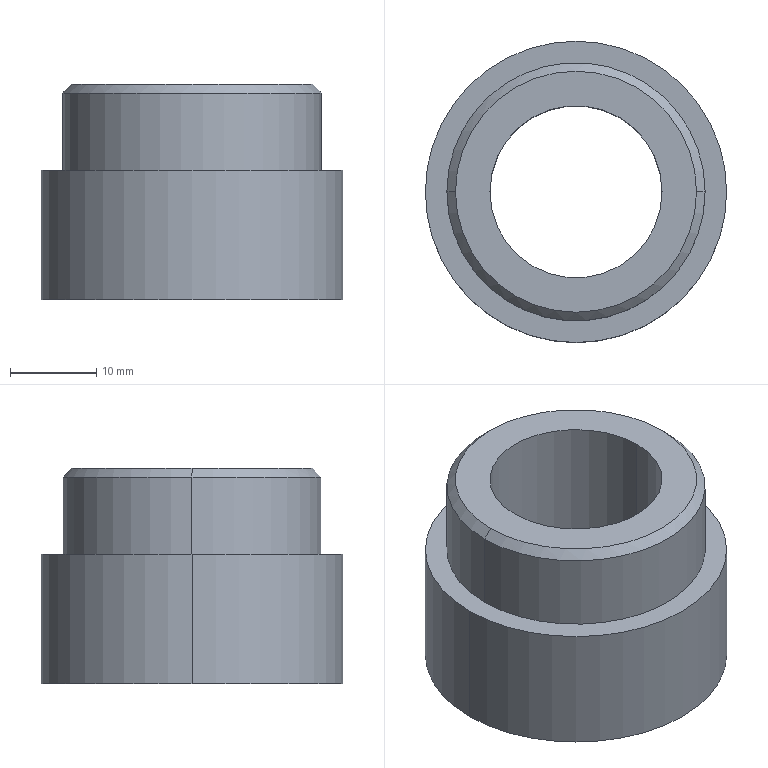Part | SolidWorks | features Chamfer 1, Extrusion 1, ICE 1 | 1 solid | 11 faces | box 35 x 35 x 25 mm | volume 13600 mm3 | cylinder 6 | plane 3 | cone 2 | commonest cylinder face diameters 20 x2 30 x2 35 x2
STEP:
#1=CARTESIAN_POINT('',(14.,0.,25.));
#2=VERTEX_POINT('',#1);
#3=CARTESIAN_POINT('',(-14.,0.,25.));
#4=VERTEX_POINT('',#3);
#5=CARTESIAN_POINT('',(0.,0.,25.));
#6=DIRECTION('',(0.,0.,1.));
#7=DIRECTION('',(1.,0.,0.));
#8=AXIS2_PLACEMENT_3D('',#5,#6,#7);
#9=CIRCLE('',#8,14.);
#10=EDGE_CURVE('',#2,#4,#9,.T.);
#11=ORIENTED_EDGE('',*,*,#10,.F.);
#12=CARTESIAN_POINT('',(15.,0.,24.));
#13=VERTEX_POINT('',#12);
#14=CARTESIAN_POINT('',(14.,0.,25.));
#15=DIRECTION('',(0.7071,0.,-0.7071));
#16=VECTOR('',#15,1000.);
#17=LINE('',#14,#16);
#18=EDGE_CURVE('',#2,#13,#17,.T.);
#19=ORIENTED_EDGE('',*,*,#18,.T.);
#20=CARTESIAN_POINT('',(-15.,0.,24.));
#21=VERTEX_POINT('',#20);
#22=CARTESIAN_POINT('',(0.,0.,24.));
#23=DIRECTION('',(0.,0.,-1.));
#24=DIRECTION('',(1.,0.,0.));
#25=AXIS2_PLACEMENT_3D('',#22,#23,#24);
#26=CIRCLE('',#25,15.);
#27=EDGE_CURVE('',#21,#13,#26,.T.);
#28=ORIENTED_EDGE('',*,*,#27,.F.);
#29=CARTESIAN_POINT('',(-14.,0.,25.));
#30=DIRECTION('',(-0.7071,0.,-0.7071));
#31=VECTOR('',#30,1000.);
#32=LINE('',#29,#31);
#33=EDGE_CURVE('',#4,#21,#32,.T.);
#34=ORIENTED_EDGE('',*,*,#33,.F.);
#35=EDGE_LOOP('',(#11,#19,#28,#34));
#36=FACE_OUTER_BOUND('',#35,.T.);
#37=CARTESIAN_POINT('',(0.,0.,25.));
#38=DIRECTION('',(0.,0.,-1.));
#39=DIRECTION('',(-1.,0.,0.));
#40=AXIS2_PLACEMENT_3D('',#37,#38,#39);
#41=CONICAL_SURFACE('',#40,14.,0.7854);
#42=ADVANCED_FACE('',(#36),#41,.T.);
#43=CARTESIAN_POINT('',(15.,0.,15.));
#44=VERTEX_POINT('',#43);
#45=CARTESIAN_POINT('',(-15.,0.,15.));
#46=VERTEX_POINT('',#45);
#47=CARTESIAN_POINT('',(0.,0.,15.));
#48=DIRECTION('',(0.,0.,1.));
#49=DIRECTION('',(1.,0.,0.));
#50=AXIS2_PLACEMENT_3D('',#47,#48,#49);
#51=CIRCLE('',#50,15.);
#52=EDGE_CURVE('',#44,#46,#51,.T.);
#53=ORIENTED_EDGE('',*,*,#52,.T.);
#54=CARTESIAN_POINT('',(-15.,0.,15.));
#55=DIRECTION('',(0.,0.,1.));
#56=VECTOR('',#55,1000.);
#57=LINE('',#54,#56);
#58=EDGE_CURVE('',#46,#21,#57,.T.);
#59=ORIENTED_EDGE('',*,*,#58,.T.);
#60=ORIENTED_EDGE('',*,*,#27,.T.);
#61=CARTESIAN_POINT('',(15.,0.,15.));
#62=DIRECTION('',(0.,0.,1.));
#63=VECTOR('',#62,1000.);
#64=LINE('',#61,#63);
#65=EDGE_CURVE('',#44,#13,#64,.T.);
#66=ORIENTED_EDGE('',*,*,#65,.F.);
#67=EDGE_LOOP('',(#53,#59,#60,#66));
#68=FACE_OUTER_BOUND('',#67,.T.);
#69=CARTESIAN_POINT('',(0.,0.,15.));
#70=DIRECTION('',(0.,0.,1.));
#71=DIRECTION('',(1.,0.,0.));
#72=AXIS2_PLACEMENT_3D('',#69,#70,#71);
#73=CYLINDRICAL_SURFACE('',#72,15.);
#74=ADVANCED_FACE('',(#68),#73,.T.);
#75=CARTESIAN_POINT('',(-10.,0.,25.));
#76=VERTEX_POINT('',#75);
#77=CARTESIAN_POINT('',(10.,0.,25.));
#78=VERTEX_POINT('',#77);
#79=CARTESIAN_POINT('',(0.,0.,25.));
#80=DIRECTION('',(0.,0.,1.));
#81=DIRECTION('',(1.,0.,0.));
#82=AXIS2_PLACEMENT_3D('',#79,#80,#81);
#83=CIRCLE('',#82,10.);
#84=EDGE_CURVE('',#76,#78,#83,.T.);
#85=ORIENTED_EDGE('',*,*,#84,.T.);
#86=CARTESIAN_POINT('',(10.,0.,0.));
#87=VERTEX_POINT('',#86);
#88=CARTESIAN_POINT('',(10.,0.,25.));
#89=DIRECTION('',(0.,0.,-1.));
#90=VECTOR('',#89,1000.);
#91=LINE('',#88,#90);
#92=EDGE_CURVE('',#78,#87,#91,.T.);
#93=ORIENTED_EDGE('',*,*,#92,.T.);
#94=CARTESIAN_POINT('',(-10.,0.,0.));
#95=VERTEX_POINT('',#94);
#96=CARTESIAN_POINT('',(0.,0.,0.));
#97=DIRECTION('',(0.,0.,1.));
#98=DIRECTION('',(1.,0.,0.));
#99=AXIS2_PLACEMENT_3D('',#96,#97,#98);
#100=CIRCLE('',#99,10.);
#101=EDGE_CURVE('',#95,#87,#100,.T.);
#102=ORIENTED_EDGE('',*,*,#101,.F.);
#103=CARTESIAN_POINT('',(-10.,0.,25.));
#104=DIRECTION('',(0.,0.,-1.));
#105=VECTOR('',#104,1000.);
#106=LINE('',#103,#105);
#107=EDGE_CURVE('',#76,#95,#106,.T.);
#108=ORIENTED_EDGE('',*,*,#107,.F.);
#109=EDGE_LOOP('',(#85,#93,#102,#108));
#110=FACE_OUTER_BOUND('',#109,.T.);
#111=CARTESIAN_POINT('',(0.,0.,25.));
#112=DIRECTION('',(0.,0.,-1.));
#113=DIRECTION('',(-1.,0.,0.));
#114=AXIS2_PLACEMENT_3D('',#111,#112,#113);
#115=CYLINDRICAL_SURFACE('',#114,10.);
#116=ADVANCED_FACE('',(#110),#115,.F.);
#117=CARTESIAN_POINT('',(17.5,0.,15.));
#118=VERTEX_POINT('',#117);
#119=CARTESIAN_POINT('',(-17.5,0.,15.));
#120=VERTEX_POINT('',#119);
#121=CARTESIAN_POINT('',(0.,0.,15.));
#122=DIRECTION('',(0.,0.,1.));
#123=DIRECTION('',(1.,0.,0.));
#124=AXIS2_PLACEMENT_3D('',#121,#122,#123);
#125=CIRCLE('',#124,17.5);
#126=EDGE_CURVE('',#118,#120,#125,.T.);
#127=ORIENTED_EDGE('',*,*,#126,.F.);
#128=CARTESIAN_POINT('',(17.5,0.,0.));
#129=VERTEX_POINT('',#128);
#130=CARTESIAN_POINT('',(17.5,0.,25.));
#131=DIRECTION('',(0.,0.,-1.));
#132=VECTOR('',#131,1000.);
#133=LINE('',#130,#132);
#134=EDGE_CURVE('',#118,#129,#133,.T.);
#135=ORIENTED_EDGE('',*,*,#134,.T.);
#136=CARTESIAN_POINT('',(-17.5,0.,0.));
#137=VERTEX_POINT('',#136);
#138=CARTESIAN_POINT('',(0.,0.,0.));
#139=DIRECTION('',(0.,0.,1.));
#140=DIRECTION('',(1.,0.,0.));
#141=AXIS2_PLACEMENT_3D('',#138,#139,#140);
#142=CIRCLE('',#141,17.5);
#143=EDGE_CURVE('',#129,#137,#142,.T.);
#144=ORIENTED_EDGE('',*,*,#143,.T.);
#145=CARTESIAN_POINT('',(-17.5,0.,25.));
#146=DIRECTION('',(0.,0.,-1.));
#147=VECTOR('',#146,1000.);
#148=LINE('',#145,#147);
#149=EDGE_CURVE('',#120,#137,#148,.T.);
#150=ORIENTED_EDGE('',*,*,#149,.F.);
#151=EDGE_LOOP('',(#127,#135,#144,#150));
#152=FACE_OUTER_BOUND('',#151,.T.);
#153=CARTESIAN_POINT('',(0.,0.,25.));
#154=DIRECTION('',(0.,0.,-1.));
#155=DIRECTION('',(-1.,0.,0.));
#156=AXIS2_PLACEMENT_3D('',#153,#154,#155);
#157=CYLINDRICAL_SURFACE('',#156,17.5);
#158=ADVANCED_FACE('',(#152),#157,.T.);
#159=CARTESIAN_POINT('',(0.,0.,25.));
#160=DIRECTION('',(0.,0.,1.));
#161=DIRECTION('',(1.,0.,0.));
#162=AXIS2_PLACEMENT_3D('',#159,#160,#161);
#163=CIRCLE('',#162,14.);
#164=EDGE_CURVE('',#4,#2,#163,.T.);
#165=ORIENTED_EDGE('',*,*,#164,.T.);
#166=ORIENTED_EDGE('',*,*,#10,.T.);
#167=EDGE_LOOP('',(#165,#166));
#168=FACE_OUTER_BOUND('',#167,.T.);
#169=ORIENTED_EDGE('',*,*,#84,.F.);
#170=CARTESIAN_POINT('',(0.,0.,25.));
#171=DIRECTION('',(0.,0.,1.));
#172=DIRECTION('',(1.,0.,0.));
#173=AXIS2_PLACEMENT_3D('',#170,#171,#172);
#174=CIRCLE('',#173,10.);
#175=EDGE_CURVE('',#78,#76,#174,.T.);
#176=ORIENTED_EDGE('',*,*,#175,.F.);
#177=EDGE_LOOP('',(#169,#176));
#178=FACE_BOUND('',#177,.T.);
#179=CARTESIAN_POINT('',(0.,0.,25.));
#180=DIRECTION('',(0.,0.,1.));
#181=DIRECTION('',(1.,0.,0.));
#182=AXIS2_PLACEMENT_3D('',#179,#180,#181);
#183=PLANE('',#182);
#184=ADVANCED_FACE('',(#168,#178),#183,.T.);
#185=ORIENTED_EDGE('',*,*,#134,.F.);
#186=CARTESIAN_POINT('',(0.,0.,15.));
#187=DIRECTION('',(0.,0.,1.));
#188=DIRECTION('',(1.,0.,0.));
#189=AXIS2_PLACEMENT_3D('',#186,#187,#188);
#190=CIRCLE('',#189,17.5);
#191=EDGE_CURVE('',#120,#118,#190,.T.);
#192=ORIENTED_EDGE('',*,*,#191,.F.);
#193=ORIENTED_EDGE('',*,*,#149,.T.);
#194=CARTESIAN_POINT('',(0.,0.,0.));
#195=DIRECTION('',(0.,0.,1.));
#196=DIRECTION('',(1.,0.,0.));
#197=AXIS2_PLACEMENT_3D('',#194,#195,#196);
#198=CIRCLE('',#197,17.5);
#199=EDGE_CURVE('',#137,#129,#198,.T.);
#200=ORIENTED_EDGE('',*,*,#199,.T.);
#201=EDGE_LOOP('',(#185,#192,#193,#200));
#202=FACE_OUTER_BOUND('',#201,.T.);
#203=CARTESIAN_POINT('',(0.,0.,25.));
#204=DIRECTION('',(0.,0.,-1.));
#205=DIRECTION('',(-1.,0.,0.));
#206=AXIS2_PLACEMENT_3D('',#203,#204,#205);
#207=CYLINDRICAL_SURFACE('',#206,17.5);
#208=ADVANCED_FACE('',(#202),#207,.T.);
#209=ORIENTED_EDGE('',*,*,#199,.F.);
#210=ORIENTED_EDGE('',*,*,#143,.F.);
#211=EDGE_LOOP('',(#209,#210));
#212=FACE_OUTER_BOUND('',#211,.T.);
#213=ORIENTED_EDGE('',*,*,#101,.T.);
#214=CARTESIAN_POINT('',(0.,0.,0.));
#215=DIRECTION('',(0.,0.,1.));
#216=DIRECTION('',(1.,0.,0.));
#217=AXIS2_PLACEMENT_3D('',#214,#215,#216);
#218=CIRCLE('',#217,10.);
#219=EDGE_CURVE('',#87,#95,#218,.T.);
#220=ORIENTED_EDGE('',*,*,#219,.T.);
#221=EDGE_LOOP('',(#213,#220));
#222=FACE_BOUND('',#221,.T.);
#223=CARTESIAN_POINT('',(0.,0.,0.));
#224=DIRECTION('',(0.,0.,1.));
#225=DIRECTION('',(1.,0.,0.));
#226=AXIS2_PLACEMENT_3D('',#223,#224,#225);
#227=PLANE('',#226);
#228=ADVANCED_FACE('',(#212,#222),#227,.F.);
#229=ORIENTED_EDGE('',*,*,#92,.F.);
#230=ORIENTED_EDGE('',*,*,#175,.T.);
#231=ORIENTED_EDGE('',*,*,#107,.T.);
#232=ORIENTED_EDGE('',*,*,#219,.F.);
#233=EDGE_LOOP('',(#229,#230,#231,#232));
#234=FACE_OUTER_BOUND('',#233,.T.);
#235=CARTESIAN_POINT('',(0.,0.,25.));
#236=DIRECTION('',(0.,0.,-1.));
#237=DIRECTION('',(-1.,0.,0.));
#238=AXIS2_PLACEMENT_3D('',#235,#236,#237);
#239=CYLINDRICAL_SURFACE('',#238,10.);
#240=ADVANCED_FACE('',(#234),#239,.F.);
#241=ORIENTED_EDGE('',*,*,#52,.F.);
#242=CARTESIAN_POINT('',(0.,0.,15.));
#243=DIRECTION('',(0.,0.,1.));
#244=DIRECTION('',(1.,0.,0.));
#245=AXIS2_PLACEMENT_3D('',#242,#243,#244);
#246=CIRCLE('',#245,15.);
#247=EDGE_CURVE('',#46,#44,#246,.T.);
#248=ORIENTED_EDGE('',*,*,#247,.F.);
#249=EDGE_LOOP('',(#241,#248));
#250=FACE_BOUND('',#249,.T.);
#251=ORIENTED_EDGE('',*,*,#191,.T.);
#252=ORIENTED_EDGE('',*,*,#126,.T.);
#253=EDGE_LOOP('',(#251,#252));
#254=FACE_OUTER_BOUND('',#253,.T.);
#255=CARTESIAN_POINT('',(0.,0.,15.));
#256=DIRECTION('',(0.,0.,1.));
#257=DIRECTION('',(1.,0.,0.));
#258=AXIS2_PLACEMENT_3D('',#255,#256,#257);
#259=PLANE('',#258);
#260=ADVANCED_FACE('',(#250,#254),#259,.T.);
#261=ORIENTED_EDGE('',*,*,#58,.F.);
#262=ORIENTED_EDGE('',*,*,#247,.T.);
#263=ORIENTED_EDGE('',*,*,#65,.T.);
#264=CARTESIAN_POINT('',(0.,0.,24.));
#265=DIRECTION('',(0.,0.,-1.));
#266=DIRECTION('',(1.,0.,0.));
#267=AXIS2_PLACEMENT_3D('',#264,#265,#266);
#268=CIRCLE('',#267,15.);
#269=EDGE_CURVE('',#13,#21,#268,.T.);
#270=ORIENTED_EDGE('',*,*,#269,.T.);
#271=EDGE_LOOP('',(#261,#262,#263,#270));
#272=FACE_OUTER_BOUND('',#271,.T.);
#273=CARTESIAN_POINT('',(0.,0.,15.));
#274=DIRECTION('',(0.,0.,1.));
#275=DIRECTION('',(1.,0.,0.));
#276=AXIS2_PLACEMENT_3D('',#273,#274,#275);
#277=CYLINDRICAL_SURFACE('',#276,15.);
#278=ADVANCED_FACE('',(#272),#277,.T.);
#279=ORIENTED_EDGE('',*,*,#18,.F.);
#280=ORIENTED_EDGE('',*,*,#164,.F.);
#281=ORIENTED_EDGE('',*,*,#33,.T.);
#282=ORIENTED_EDGE('',*,*,#269,.F.);
#283=EDGE_LOOP('',(#279,#280,#281,#282));
#284=FACE_OUTER_BOUND('',#283,.T.);
#285=CARTESIAN_POINT('',(0.,0.,25.));
#286=DIRECTION('',(0.,0.,-1.));
#287=DIRECTION('',(-1.,0.,0.));
#288=AXIS2_PLACEMENT_3D('',#285,#286,#287);
#289=CONICAL_SURFACE('',#288,14.,0.7854);
#290=ADVANCED_FACE('',(#284),#289,.T.);
#291=CLOSED_SHELL('',(#42,#74,#116,#158,#184,#208,#228,#240,#260,#278,#290));
#292=MANIFOLD_SOLID_BREP('',#291);
#293=CARTESIAN_POINT('',(0.,0.,0.));
#294=DIRECTION('',(0.,0.,1.));
#295=DIRECTION('',(1.,0.,0.));
#296=AXIS2_PLACEMENT_3D('',#293,#294,#295);
#297=(LENGTH_UNIT()NAMED_UNIT(*)SI_UNIT(.MILLI.,.METRE.));
#298=UNCERTAINTY_MEASURE_WITH_UNIT(LENGTH_MEASURE(0.00001),#297,'','');
#299=(NAMED_UNIT(*)PLANE_ANGLE_UNIT()SI_UNIT($,.RADIAN.));
#300=(NAMED_UNIT(*)SI_UNIT($,.STERADIAN.)SOLID_ANGLE_UNIT());
#301=(GEOMETRIC_REPRESENTATION_CONTEXT(3)GLOBAL_UNCERTAINTY_ASSIGNED_CONTEXT((#298))GLOBAL_UNIT_ASSIGNED_CONTEXT((#297,#299,#300))REPRESENTATION_CONTEXT('',''));
#302=ADVANCED_BREP_SHAPE_REPRESENTATION('',(#292,#296),#301);